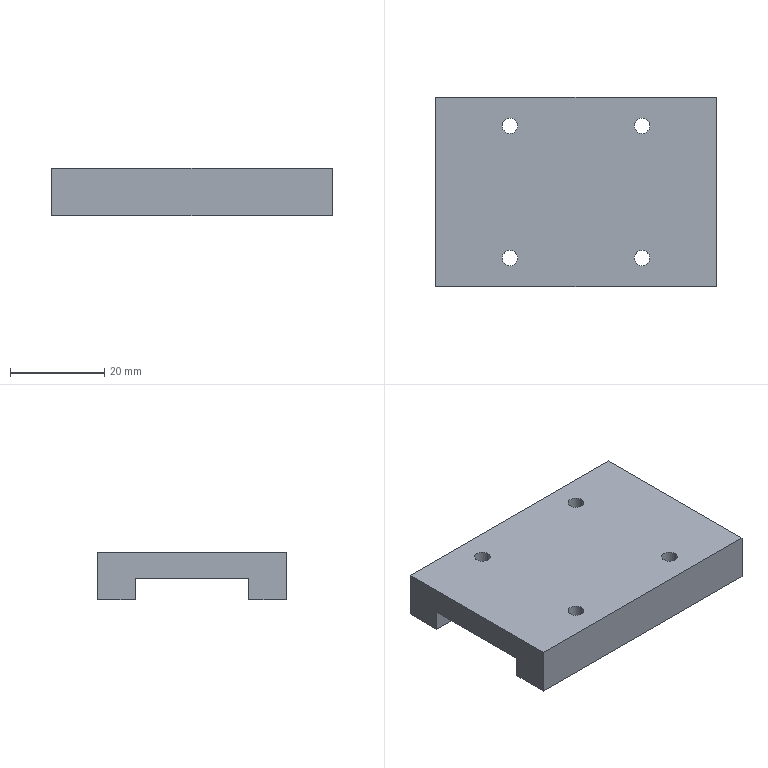Part | SolidWorks | features Extrusion 1, HoleWzd 1, ICE 1 | 1 solid | 18 faces | box 59.4 x 40 x 10 mm | volume 17003 mm3 | plane 10 | cylinder 8 | commonest cylinder face diameters 3.3 x8
STEP:
#1=CARTESIAN_POINT('',(-15.65,14.,0.));
#2=VERTEX_POINT('',#1);
#3=CARTESIAN_POINT('',(-12.35,14.,0.));
#4=VERTEX_POINT('',#3);
#5=CARTESIAN_POINT('',(-14.,14.,0.));
#6=DIRECTION('',(0.,0.,1.));
#7=DIRECTION('',(1.,0.,0.));
#8=AXIS2_PLACEMENT_3D('',#5,#6,#7);
#9=CIRCLE('',#8,1.65);
#10=EDGE_CURVE('',#2,#4,#9,.T.);
#11=ORIENTED_EDGE('',*,*,#10,.F.);
#12=CARTESIAN_POINT('',(-15.65,14.,10.));
#13=VERTEX_POINT('',#12);
#14=CARTESIAN_POINT('',(-15.65,14.,10.));
#15=DIRECTION('',(0.,0.,1.));
#16=VECTOR('',#15,1000.);
#17=LINE('',#14,#16);
#18=EDGE_CURVE('',#2,#13,#17,.T.);
#19=ORIENTED_EDGE('',*,*,#18,.T.);
#20=CARTESIAN_POINT('',(-12.35,14.,10.));
#21=VERTEX_POINT('',#20);
#22=CARTESIAN_POINT('',(-14.,14.,10.));
#23=DIRECTION('',(0.,0.,1.));
#24=DIRECTION('',(1.,0.,0.));
#25=AXIS2_PLACEMENT_3D('',#22,#23,#24);
#26=CIRCLE('',#25,1.65);
#27=EDGE_CURVE('',#13,#21,#26,.T.);
#28=ORIENTED_EDGE('',*,*,#27,.T.);
#29=CARTESIAN_POINT('',(-12.35,14.,10.));
#30=DIRECTION('',(0.,0.,1.));
#31=VECTOR('',#30,1000.);
#32=LINE('',#29,#31);
#33=EDGE_CURVE('',#4,#21,#32,.T.);
#34=ORIENTED_EDGE('',*,*,#33,.F.);
#35=EDGE_LOOP('',(#11,#19,#28,#34));
#36=FACE_OUTER_BOUND('',#35,.T.);
#37=CARTESIAN_POINT('',(-14.,14.,10.));
#38=DIRECTION('',(0.,0.,1.));
#39=DIRECTION('',(1.,0.,0.));
#40=AXIS2_PLACEMENT_3D('',#37,#38,#39);
#41=CYLINDRICAL_SURFACE('',#40,1.65);
#42=ADVANCED_FACE('',(#36),#41,.F.);
#43=CARTESIAN_POINT('',(12.35,14.,0.));
#44=VERTEX_POINT('',#43);
#45=CARTESIAN_POINT('',(15.65,14.,0.));
#46=VERTEX_POINT('',#45);
#47=CARTESIAN_POINT('',(14.,14.,0.));
#48=DIRECTION('',(0.,0.,1.));
#49=DIRECTION('',(1.,0.,0.));
#50=AXIS2_PLACEMENT_3D('',#47,#48,#49);
#51=CIRCLE('',#50,1.65);
#52=EDGE_CURVE('',#44,#46,#51,.T.);
#53=ORIENTED_EDGE('',*,*,#52,.F.);
#54=CARTESIAN_POINT('',(12.35,14.,10.));
#55=VERTEX_POINT('',#54);
#56=CARTESIAN_POINT('',(12.35,14.,10.));
#57=DIRECTION('',(0.,0.,1.));
#58=VECTOR('',#57,1000.);
#59=LINE('',#56,#58);
#60=EDGE_CURVE('',#44,#55,#59,.T.);
#61=ORIENTED_EDGE('',*,*,#60,.T.);
#62=CARTESIAN_POINT('',(15.65,14.,10.));
#63=VERTEX_POINT('',#62);
#64=CARTESIAN_POINT('',(14.,14.,10.));
#65=DIRECTION('',(0.,0.,1.));
#66=DIRECTION('',(1.,0.,0.));
#67=AXIS2_PLACEMENT_3D('',#64,#65,#66);
#68=CIRCLE('',#67,1.65);
#69=EDGE_CURVE('',#55,#63,#68,.T.);
#70=ORIENTED_EDGE('',*,*,#69,.T.);
#71=CARTESIAN_POINT('',(15.65,14.,10.));
#72=DIRECTION('',(0.,0.,1.));
#73=VECTOR('',#72,1000.);
#74=LINE('',#71,#73);
#75=EDGE_CURVE('',#46,#63,#74,.T.);
#76=ORIENTED_EDGE('',*,*,#75,.F.);
#77=EDGE_LOOP('',(#53,#61,#70,#76));
#78=FACE_OUTER_BOUND('',#77,.T.);
#79=CARTESIAN_POINT('',(14.,14.,10.));
#80=DIRECTION('',(0.,0.,1.));
#81=DIRECTION('',(1.,0.,0.));
#82=AXIS2_PLACEMENT_3D('',#79,#80,#81);
#83=CYLINDRICAL_SURFACE('',#82,1.65);
#84=ADVANCED_FACE('',(#78),#83,.F.);
#85=CARTESIAN_POINT('',(12.35,-14.,0.));
#86=VERTEX_POINT('',#85);
#87=CARTESIAN_POINT('',(15.65,-14.,0.));
#88=VERTEX_POINT('',#87);
#89=CARTESIAN_POINT('',(14.,-14.,0.));
#90=DIRECTION('',(0.,0.,1.));
#91=DIRECTION('',(1.,0.,0.));
#92=AXIS2_PLACEMENT_3D('',#89,#90,#91);
#93=CIRCLE('',#92,1.65);
#94=EDGE_CURVE('',#86,#88,#93,.T.);
#95=ORIENTED_EDGE('',*,*,#94,.F.);
#96=CARTESIAN_POINT('',(12.35,-14.,10.));
#97=VERTEX_POINT('',#96);
#98=CARTESIAN_POINT('',(12.35,-14.,10.));
#99=DIRECTION('',(0.,0.,1.));
#100=VECTOR('',#99,1000.);
#101=LINE('',#98,#100);
#102=EDGE_CURVE('',#86,#97,#101,.T.);
#103=ORIENTED_EDGE('',*,*,#102,.T.);
#104=CARTESIAN_POINT('',(15.65,-14.,10.));
#105=VERTEX_POINT('',#104);
#106=CARTESIAN_POINT('',(14.,-14.,10.));
#107=DIRECTION('',(0.,0.,1.));
#108=DIRECTION('',(1.,0.,0.));
#109=AXIS2_PLACEMENT_3D('',#106,#107,#108);
#110=CIRCLE('',#109,1.65);
#111=EDGE_CURVE('',#97,#105,#110,.T.);
#112=ORIENTED_EDGE('',*,*,#111,.T.);
#113=CARTESIAN_POINT('',(15.65,-14.,10.));
#114=DIRECTION('',(0.,0.,1.));
#115=VECTOR('',#114,1000.);
#116=LINE('',#113,#115);
#117=EDGE_CURVE('',#88,#105,#116,.T.);
#118=ORIENTED_EDGE('',*,*,#117,.F.);
#119=EDGE_LOOP('',(#95,#103,#112,#118));
#120=FACE_OUTER_BOUND('',#119,.T.);
#121=CARTESIAN_POINT('',(14.,-14.,10.));
#122=DIRECTION('',(0.,0.,1.));
#123=DIRECTION('',(1.,0.,0.));
#124=AXIS2_PLACEMENT_3D('',#121,#122,#123);
#125=CYLINDRICAL_SURFACE('',#124,1.65);
#126=ADVANCED_FACE('',(#120),#125,.F.);
#127=CARTESIAN_POINT('',(-15.65,-14.,0.));
#128=VERTEX_POINT('',#127);
#129=CARTESIAN_POINT('',(-12.35,-14.,0.));
#130=VERTEX_POINT('',#129);
#131=CARTESIAN_POINT('',(-14.,-14.,0.));
#132=DIRECTION('',(0.,0.,1.));
#133=DIRECTION('',(1.,0.,0.));
#134=AXIS2_PLACEMENT_3D('',#131,#132,#133);
#135=CIRCLE('',#134,1.65);
#136=EDGE_CURVE('',#128,#130,#135,.T.);
#137=ORIENTED_EDGE('',*,*,#136,.F.);
#138=CARTESIAN_POINT('',(-15.65,-14.,10.));
#139=VERTEX_POINT('',#138);
#140=CARTESIAN_POINT('',(-15.65,-14.,10.));
#141=DIRECTION('',(0.,0.,1.));
#142=VECTOR('',#141,1000.);
#143=LINE('',#140,#142);
#144=EDGE_CURVE('',#128,#139,#143,.T.);
#145=ORIENTED_EDGE('',*,*,#144,.T.);
#146=CARTESIAN_POINT('',(-12.35,-14.,10.));
#147=VERTEX_POINT('',#146);
#148=CARTESIAN_POINT('',(-14.,-14.,10.));
#149=DIRECTION('',(0.,0.,1.));
#150=DIRECTION('',(1.,0.,0.));
#151=AXIS2_PLACEMENT_3D('',#148,#149,#150);
#152=CIRCLE('',#151,1.65);
#153=EDGE_CURVE('',#139,#147,#152,.T.);
#154=ORIENTED_EDGE('',*,*,#153,.T.);
#155=CARTESIAN_POINT('',(-12.35,-14.,10.));
#156=DIRECTION('',(0.,0.,1.));
#157=VECTOR('',#156,1000.);
#158=LINE('',#155,#157);
#159=EDGE_CURVE('',#130,#147,#158,.T.);
#160=ORIENTED_EDGE('',*,*,#159,.F.);
#161=EDGE_LOOP('',(#137,#145,#154,#160));
#162=FACE_OUTER_BOUND('',#161,.T.);
#163=CARTESIAN_POINT('',(-14.,-14.,10.));
#164=DIRECTION('',(0.,0.,1.));
#165=DIRECTION('',(1.,0.,0.));
#166=AXIS2_PLACEMENT_3D('',#163,#164,#165);
#167=CYLINDRICAL_SURFACE('',#166,1.65);
#168=ADVANCED_FACE('',(#162),#167,.F.);
#169=CARTESIAN_POINT('',(14.,-14.,0.));
#170=DIRECTION('',(0.,0.,1.));
#171=DIRECTION('',(1.,0.,0.));
#172=AXIS2_PLACEMENT_3D('',#169,#170,#171);
#173=CIRCLE('',#172,1.65);
#174=EDGE_CURVE('',#88,#86,#173,.T.);
#175=ORIENTED_EDGE('',*,*,#174,.T.);
#176=ORIENTED_EDGE('',*,*,#94,.T.);
#177=EDGE_LOOP('',(#175,#176));
#178=FACE_BOUND('',#177,.T.);
#179=CARTESIAN_POINT('',(-14.,-14.,0.));
#180=DIRECTION('',(0.,0.,1.));
#181=DIRECTION('',(1.,0.,0.));
#182=AXIS2_PLACEMENT_3D('',#179,#180,#181);
#183=CIRCLE('',#182,1.65);
#184=EDGE_CURVE('',#130,#128,#183,.T.);
#185=ORIENTED_EDGE('',*,*,#184,.T.);
#186=ORIENTED_EDGE('',*,*,#136,.T.);
#187=EDGE_LOOP('',(#185,#186));
#188=FACE_BOUND('',#187,.T.);
#189=CARTESIAN_POINT('',(-29.7,-12.,0.));
#190=VERTEX_POINT('',#189);
#191=CARTESIAN_POINT('',(-29.7,-20.,0.));
#192=VERTEX_POINT('',#191);
#193=CARTESIAN_POINT('',(-29.7,20.,0.));
#194=DIRECTION('',(0.,-1.,0.));
#195=VECTOR('',#194,1000.);
#196=LINE('',#193,#195);
#197=EDGE_CURVE('',#190,#192,#196,.T.);
#198=ORIENTED_EDGE('',*,*,#197,.F.);
#199=CARTESIAN_POINT('',(29.7,-12.,0.));
#200=VERTEX_POINT('',#199);
#201=CARTESIAN_POINT('',(0.,-12.,0.));
#202=DIRECTION('',(1.,0.,0.));
#203=VECTOR('',#202,1000.);
#204=LINE('',#201,#203);
#205=EDGE_CURVE('',#190,#200,#204,.T.);
#206=ORIENTED_EDGE('',*,*,#205,.T.);
#207=CARTESIAN_POINT('',(29.7,-20.,0.));
#208=VERTEX_POINT('',#207);
#209=CARTESIAN_POINT('',(29.7,20.,0.));
#210=DIRECTION('',(0.,1.,0.));
#211=VECTOR('',#210,1000.);
#212=LINE('',#209,#211);
#213=EDGE_CURVE('',#208,#200,#212,.T.);
#214=ORIENTED_EDGE('',*,*,#213,.F.);
#215=CARTESIAN_POINT('',(-29.7,-20.,0.));
#216=DIRECTION('',(1.,0.,0.));
#217=VECTOR('',#216,1000.);
#218=LINE('',#215,#217);
#219=EDGE_CURVE('',#192,#208,#218,.T.);
#220=ORIENTED_EDGE('',*,*,#219,.F.);
#221=EDGE_LOOP('',(#198,#206,#214,#220));
#222=FACE_OUTER_BOUND('',#221,.T.);
#223=CARTESIAN_POINT('',(0.,0.,0.));
#224=DIRECTION('',(0.,0.,1.));
#225=DIRECTION('',(1.,0.,0.));
#226=AXIS2_PLACEMENT_3D('',#223,#224,#225);
#227=PLANE('',#226);
#228=ADVANCED_FACE('',(#178,#188,#222),#227,.F.);
#229=ORIENTED_EDGE('',*,*,#213,.T.);
#230=CARTESIAN_POINT('',(29.7,-12.,4.5));
#231=VERTEX_POINT('',#230);
#232=CARTESIAN_POINT('',(29.7,-12.,-4.5));
#233=DIRECTION('',(0.,0.,1.));
#234=VECTOR('',#233,1000.);
#235=LINE('',#232,#234);
#236=EDGE_CURVE('',#200,#231,#235,.T.);
#237=ORIENTED_EDGE('',*,*,#236,.T.);
#238=CARTESIAN_POINT('',(29.7,12.,4.5));
#239=VERTEX_POINT('',#238);
#240=CARTESIAN_POINT('',(29.7,12.,4.5));
#241=DIRECTION('',(0.,1.,0.));
#242=VECTOR('',#241,1000.);
#243=LINE('',#240,#242);
#244=EDGE_CURVE('',#231,#239,#243,.T.);
#245=ORIENTED_EDGE('',*,*,#244,.T.);
#246=CARTESIAN_POINT('',(29.7,12.,0.));
#247=VERTEX_POINT('',#246);
#248=CARTESIAN_POINT('',(29.7,12.,-4.5));
#249=DIRECTION('',(0.,0.,-1.));
#250=VECTOR('',#249,1000.);
#251=LINE('',#248,#250);
#252=EDGE_CURVE('',#239,#247,#251,.T.);
#253=ORIENTED_EDGE('',*,*,#252,.T.);
#254=CARTESIAN_POINT('',(29.7,20.,0.));
#255=VERTEX_POINT('',#254);
#256=CARTESIAN_POINT('',(29.7,20.,0.));
#257=DIRECTION('',(0.,1.,0.));
#258=VECTOR('',#257,1000.);
#259=LINE('',#256,#258);
#260=EDGE_CURVE('',#247,#255,#259,.T.);
#261=ORIENTED_EDGE('',*,*,#260,.T.);
#262=CARTESIAN_POINT('',(29.7,20.,10.));
#263=VERTEX_POINT('',#262);
#264=CARTESIAN_POINT('',(29.7,20.,10.));
#265=DIRECTION('',(0.,0.,-1.));
#266=VECTOR('',#265,1000.);
#267=LINE('',#264,#266);
#268=EDGE_CURVE('',#263,#255,#267,.T.);
#269=ORIENTED_EDGE('',*,*,#268,.F.);
#270=CARTESIAN_POINT('',(29.7,-20.,10.));
#271=VERTEX_POINT('',#270);
#272=CARTESIAN_POINT('',(29.7,20.,10.));
#273=DIRECTION('',(0.,1.,0.));
#274=VECTOR('',#273,1000.);
#275=LINE('',#272,#274);
#276=EDGE_CURVE('',#271,#263,#275,.T.);
#277=ORIENTED_EDGE('',*,*,#276,.F.);
#278=CARTESIAN_POINT('',(29.7,-20.,10.));
#279=DIRECTION('',(0.,0.,-1.));
#280=VECTOR('',#279,1000.);
#281=LINE('',#278,#280);
#282=EDGE_CURVE('',#271,#208,#281,.T.);
#283=ORIENTED_EDGE('',*,*,#282,.T.);
#284=EDGE_LOOP('',(#229,#237,#245,#253,#261,#269,#277,#283));
#285=FACE_OUTER_BOUND('',#284,.T.);
#286=CARTESIAN_POINT('',(29.7,20.,10.));
#287=DIRECTION('',(-1.,0.,0.));
#288=DIRECTION('',(0.,-1.,0.));
#289=AXIS2_PLACEMENT_3D('',#286,#287,#288);
#290=PLANE('',#289);
#291=ADVANCED_FACE('',(#285),#290,.F.);
#292=CARTESIAN_POINT('',(-29.7,20.,0.));
#293=VERTEX_POINT('',#292);
#294=CARTESIAN_POINT('',(-29.7,20.,0.));
#295=DIRECTION('',(-1.,0.,0.));
#296=VECTOR('',#295,1000.);
#297=LINE('',#294,#296);
#298=EDGE_CURVE('',#255,#293,#297,.T.);
#299=ORIENTED_EDGE('',*,*,#298,.T.);
#300=CARTESIAN_POINT('',(-29.7,20.,10.));
#301=VERTEX_POINT('',#300);
#302=CARTESIAN_POINT('',(-29.7,20.,10.));
#303=DIRECTION('',(0.,0.,-1.));
#304=VECTOR('',#303,1000.);
#305=LINE('',#302,#304);
#306=EDGE_CURVE('',#301,#293,#305,.T.);
#307=ORIENTED_EDGE('',*,*,#306,.F.);
#308=CARTESIAN_POINT('',(-29.7,20.,10.));
#309=DIRECTION('',(-1.,0.,0.));
#310=VECTOR('',#309,1000.);
#311=LINE('',#308,#310);
#312=EDGE_CURVE('',#263,#301,#311,.T.);
#313=ORIENTED_EDGE('',*,*,#312,.F.);
#314=ORIENTED_EDGE('',*,*,#268,.T.);
#315=EDGE_LOOP('',(#299,#307,#313,#314));
#316=FACE_OUTER_BOUND('',#315,.T.);
#317=CARTESIAN_POINT('',(-29.7,20.,10.));
#318=DIRECTION('',(0.,-1.,0.));
#319=DIRECTION('',(0.,0.,-1.));
#320=AXIS2_PLACEMENT_3D('',#317,#318,#319);
#321=PLANE('',#320);
#322=ADVANCED_FACE('',(#316),#321,.F.);
#323=CARTESIAN_POINT('',(-29.7,-12.,4.5));
#324=VERTEX_POINT('',#323);
#325=CARTESIAN_POINT('',(-29.7,12.,4.5));
#326=VERTEX_POINT('',#325);
#327=CARTESIAN_POINT('',(-29.7,12.,4.5));
#328=DIRECTION('',(0.,1.,0.));
#329=VECTOR('',#328,1000.);
#330=LINE('',#327,#329);
#331=EDGE_CURVE('',#324,#326,#330,.T.);
#332=ORIENTED_EDGE('',*,*,#331,.F.);
#333=CARTESIAN_POINT('',(-29.7,-12.,-4.5));
#334=DIRECTION('',(0.,0.,1.));
#335=VECTOR('',#334,1000.);
#336=LINE('',#333,#335);
#337=EDGE_CURVE('',#190,#324,#336,.T.);
#338=ORIENTED_EDGE('',*,*,#337,.F.);
#339=ORIENTED_EDGE('',*,*,#197,.T.);
#340=CARTESIAN_POINT('',(-29.7,-20.,10.));
#341=VERTEX_POINT('',#340);
#342=CARTESIAN_POINT('',(-29.7,-20.,10.));
#343=DIRECTION('',(0.,0.,-1.));
#344=VECTOR('',#343,1000.);
#345=LINE('',#342,#344);
#346=EDGE_CURVE('',#341,#192,#345,.T.);
#347=ORIENTED_EDGE('',*,*,#346,.F.);
#348=CARTESIAN_POINT('',(-29.7,20.,10.));
#349=DIRECTION('',(0.,-1.,0.));
#350=VECTOR('',#349,1000.);
#351=LINE('',#348,#350);
#352=EDGE_CURVE('',#301,#341,#351,.T.);
#353=ORIENTED_EDGE('',*,*,#352,.F.);
#354=ORIENTED_EDGE('',*,*,#306,.T.);
#355=CARTESIAN_POINT('',(-29.7,12.,0.));
#356=VERTEX_POINT('',#355);
#357=CARTESIAN_POINT('',(-29.7,20.,0.));
#358=DIRECTION('',(0.,-1.,0.));
#359=VECTOR('',#358,1000.);
#360=LINE('',#357,#359);
#361=EDGE_CURVE('',#293,#356,#360,.T.);
#362=ORIENTED_EDGE('',*,*,#361,.T.);
#363=CARTESIAN_POINT('',(-29.7,12.,-4.5));
#364=DIRECTION('',(0.,0.,-1.));
#365=VECTOR('',#364,1000.);
#366=LINE('',#363,#365);
#367=EDGE_CURVE('',#326,#356,#366,.T.);
#368=ORIENTED_EDGE('',*,*,#367,.F.);
#369=EDGE_LOOP('',(#332,#338,#339,#347,#353,#354,#362,#368));
#370=FACE_OUTER_BOUND('',#369,.T.);
#371=CARTESIAN_POINT('',(-29.7,20.,10.));
#372=DIRECTION('',(1.,0.,0.));
#373=DIRECTION('',(0.,1.,0.));
#374=AXIS2_PLACEMENT_3D('',#371,#372,#373);
#375=PLANE('',#374);
#376=ADVANCED_FACE('',(#370),#375,.F.);
#377=ORIENTED_EDGE('',*,*,#219,.T.);
#378=ORIENTED_EDGE('',*,*,#282,.F.);
#379=CARTESIAN_POINT('',(-29.7,-20.,10.));
#380=DIRECTION('',(1.,0.,0.));
#381=VECTOR('',#380,1000.);
#382=LINE('',#379,#381);
#383=EDGE_CURVE('',#341,#271,#382,.T.);
#384=ORIENTED_EDGE('',*,*,#383,.F.);
#385=ORIENTED_EDGE('',*,*,#346,.T.);
#386=EDGE_LOOP('',(#377,#378,#384,#385));
#387=FACE_OUTER_BOUND('',#386,.T.);
#388=CARTESIAN_POINT('',(-29.7,-20.,10.));
#389=DIRECTION('',(0.,1.,0.));
#390=DIRECTION('',(0.,0.,1.));
#391=AXIS2_PLACEMENT_3D('',#388,#389,#390);
#392=PLANE('',#391);
#393=ADVANCED_FACE('',(#387),#392,.F.);
#394=CARTESIAN_POINT('',(-14.,14.,10.));
#395=DIRECTION('',(0.,0.,1.));
#396=DIRECTION('',(1.,0.,0.));
#397=AXIS2_PLACEMENT_3D('',#394,#395,#396);
#398=CIRCLE('',#397,1.65);
#399=EDGE_CURVE('',#21,#13,#398,.T.);
#400=ORIENTED_EDGE('',*,*,#399,.F.);
#401=ORIENTED_EDGE('',*,*,#27,.F.);
#402=EDGE_LOOP('',(#400,#401));
#403=FACE_BOUND('',#402,.T.);
#404=CARTESIAN_POINT('',(14.,14.,10.));
#405=DIRECTION('',(0.,0.,1.));
#406=DIRECTION('',(1.,0.,0.));
#407=AXIS2_PLACEMENT_3D('',#404,#405,#406);
#408=CIRCLE('',#407,1.65);
#409=EDGE_CURVE('',#63,#55,#408,.T.);
#410=ORIENTED_EDGE('',*,*,#409,.F.);
#411=ORIENTED_EDGE('',*,*,#69,.F.);
#412=EDGE_LOOP('',(#410,#411));
#413=FACE_BOUND('',#412,.T.);
#414=CARTESIAN_POINT('',(14.,-14.,10.));
#415=DIRECTION('',(0.,0.,1.));
#416=DIRECTION('',(1.,0.,0.));
#417=AXIS2_PLACEMENT_3D('',#414,#415,#416);
#418=CIRCLE('',#417,1.65);
#419=EDGE_CURVE('',#105,#97,#418,.T.);
#420=ORIENTED_EDGE('',*,*,#419,.F.);
#421=ORIENTED_EDGE('',*,*,#111,.F.);
#422=EDGE_LOOP('',(#420,#421));
#423=FACE_BOUND('',#422,.T.);
#424=CARTESIAN_POINT('',(-14.,-14.,10.));
#425=DIRECTION('',(0.,0.,1.));
#426=DIRECTION('',(1.,0.,0.));
#427=AXIS2_PLACEMENT_3D('',#424,#425,#426);
#428=CIRCLE('',#427,1.65);
#429=EDGE_CURVE('',#147,#139,#428,.T.);
#430=ORIENTED_EDGE('',*,*,#429,.F.);
#431=ORIENTED_EDGE('',*,*,#153,.F.);
#432=EDGE_LOOP('',(#430,#431));
#433=FACE_BOUND('',#432,.T.);
#434=ORIENTED_EDGE('',*,*,#276,.T.);
#435=ORIENTED_EDGE('',*,*,#312,.T.);
#436=ORIENTED_EDGE('',*,*,#352,.T.);
#437=ORIENTED_EDGE('',*,*,#383,.T.);
#438=EDGE_LOOP('',(#434,#435,#436,#437));
#439=FACE_OUTER_BOUND('',#438,.T.);
#440=CARTESIAN_POINT('',(0.,0.,10.));
#441=DIRECTION('',(0.,0.,1.));
#442=DIRECTION('',(1.,0.,0.));
#443=AXIS2_PLACEMENT_3D('',#440,#441,#442);
#444=PLANE('',#443);
#445=ADVANCED_FACE('',(#403,#413,#423,#433,#439),#444,.T.);
#446=CARTESIAN_POINT('',(-14.,14.,0.));
#447=DIRECTION('',(0.,0.,1.));
#448=DIRECTION('',(1.,0.,0.));
#449=AXIS2_PLACEMENT_3D('',#446,#447,#448);
#450=CIRCLE('',#449,1.65);
#451=EDGE_CURVE('',#4,#2,#450,.T.);
#452=ORIENTED_EDGE('',*,*,#451,.T.);
#453=ORIENTED_EDGE('',*,*,#10,.T.);
#454=EDGE_LOOP('',(#452,#453));
#455=FACE_BOUND('',#454,.T.);
#456=CARTESIAN_POINT('',(14.,14.,0.));
#457=DIRECTION('',(0.,0.,1.));
#458=DIRECTION('',(1.,0.,0.));
#459=AXIS2_PLACEMENT_3D('',#456,#457,#458);
#460=CIRCLE('',#459,1.65);
#461=EDGE_CURVE('',#46,#44,#460,.T.);
#462=ORIENTED_EDGE('',*,*,#461,.T.);
#463=ORIENTED_EDGE('',*,*,#52,.T.);
#464=EDGE_LOOP('',(#462,#463));
#465=FACE_BOUND('',#464,.T.);
#466=ORIENTED_EDGE('',*,*,#260,.F.);
#467=CARTESIAN_POINT('',(0.,12.,0.));
#468=DIRECTION('',(-1.,0.,0.));
#469=VECTOR('',#468,1000.);
#470=LINE('',#467,#469);
#471=EDGE_CURVE('',#247,#356,#470,.T.);
#472=ORIENTED_EDGE('',*,*,#471,.T.);
#473=ORIENTED_EDGE('',*,*,#361,.F.);
#474=ORIENTED_EDGE('',*,*,#298,.F.);
#475=EDGE_LOOP('',(#466,#472,#473,#474));
#476=FACE_OUTER_BOUND('',#475,.T.);
#477=CARTESIAN_POINT('',(0.,0.,0.));
#478=DIRECTION('',(0.,0.,1.));
#479=DIRECTION('',(1.,0.,0.));
#480=AXIS2_PLACEMENT_3D('',#477,#478,#479);
#481=PLANE('',#480);
#482=ADVANCED_FACE('',(#455,#465,#476),#481,.F.);
#483=ORIENTED_EDGE('',*,*,#337,.T.);
#484=CARTESIAN_POINT('',(29.7,-12.,4.5));
#485=DIRECTION('',(-1.,0.,0.));
#486=VECTOR('',#485,1000.);
#487=LINE('',#484,#486);
#488=EDGE_CURVE('',#231,#324,#487,.T.);
#489=ORIENTED_EDGE('',*,*,#488,.F.);
#490=ORIENTED_EDGE('',*,*,#236,.F.);
#491=ORIENTED_EDGE('',*,*,#205,.F.);
#492=EDGE_LOOP('',(#483,#489,#490,#491));
#493=FACE_OUTER_BOUND('',#492,.T.);
#494=CARTESIAN_POINT('',(29.7,-12.,-4.5));
#495=DIRECTION('',(0.,-1.,0.));
#496=DIRECTION('',(1.,0.,0.));
#497=AXIS2_PLACEMENT_3D('',#494,#495,#496);
#498=PLANE('',#497);
#499=ADVANCED_FACE('',(#493),#498,.F.);
#500=ORIENTED_EDGE('',*,*,#252,.F.);
#501=CARTESIAN_POINT('',(29.7,12.,4.5));
#502=DIRECTION('',(-1.,0.,0.));
#503=VECTOR('',#502,1000.);
#504=LINE('',#501,#503);
#505=EDGE_CURVE('',#239,#326,#504,.T.);
#506=ORIENTED_EDGE('',*,*,#505,.T.);
#507=ORIENTED_EDGE('',*,*,#367,.T.);
#508=ORIENTED_EDGE('',*,*,#471,.F.);
#509=EDGE_LOOP('',(#500,#506,#507,#508));
#510=FACE_OUTER_BOUND('',#509,.T.);
#511=CARTESIAN_POINT('',(29.7,12.,-4.5));
#512=DIRECTION('',(0.,1.,0.));
#513=DIRECTION('',(-1.,0.,0.));
#514=AXIS2_PLACEMENT_3D('',#511,#512,#513);
#515=PLANE('',#514);
#516=ADVANCED_FACE('',(#510),#515,.F.);
#517=ORIENTED_EDGE('',*,*,#331,.T.);
#518=ORIENTED_EDGE('',*,*,#505,.F.);
#519=ORIENTED_EDGE('',*,*,#244,.F.);
#520=ORIENTED_EDGE('',*,*,#488,.T.);
#521=EDGE_LOOP('',(#517,#518,#519,#520));
#522=FACE_OUTER_BOUND('',#521,.T.);
#523=CARTESIAN_POINT('',(29.7,12.,4.5));
#524=DIRECTION('',(0.,0.,1.));
#525=DIRECTION('',(1.,0.,0.));
#526=AXIS2_PLACEMENT_3D('',#523,#524,#525);
#527=PLANE('',#526);
#528=ADVANCED_FACE('',(#522),#527,.F.);
#529=ORIENTED_EDGE('',*,*,#144,.F.);
#530=ORIENTED_EDGE('',*,*,#184,.F.);
#531=ORIENTED_EDGE('',*,*,#159,.T.);
#532=ORIENTED_EDGE('',*,*,#429,.T.);
#533=EDGE_LOOP('',(#529,#530,#531,#532));
#534=FACE_OUTER_BOUND('',#533,.T.);
#535=CARTESIAN_POINT('',(-14.,-14.,10.));
#536=DIRECTION('',(0.,0.,1.));
#537=DIRECTION('',(1.,0.,0.));
#538=AXIS2_PLACEMENT_3D('',#535,#536,#537);
#539=CYLINDRICAL_SURFACE('',#538,1.65);
#540=ADVANCED_FACE('',(#534),#539,.F.);
#541=ORIENTED_EDGE('',*,*,#102,.F.);
#542=ORIENTED_EDGE('',*,*,#174,.F.);
#543=ORIENTED_EDGE('',*,*,#117,.T.);
#544=ORIENTED_EDGE('',*,*,#419,.T.);
#545=EDGE_LOOP('',(#541,#542,#543,#544));
#546=FACE_OUTER_BOUND('',#545,.T.);
#547=CARTESIAN_POINT('',(14.,-14.,10.));
#548=DIRECTION('',(0.,0.,1.));
#549=DIRECTION('',(1.,0.,0.));
#550=AXIS2_PLACEMENT_3D('',#547,#548,#549);
#551=CYLINDRICAL_SURFACE('',#550,1.65);
#552=ADVANCED_FACE('',(#546),#551,.F.);
#553=ORIENTED_EDGE('',*,*,#60,.F.);
#554=ORIENTED_EDGE('',*,*,#461,.F.);
#555=ORIENTED_EDGE('',*,*,#75,.T.);
#556=ORIENTED_EDGE('',*,*,#409,.T.);
#557=EDGE_LOOP('',(#553,#554,#555,#556));
#558=FACE_OUTER_BOUND('',#557,.T.);
#559=CARTESIAN_POINT('',(14.,14.,10.));
#560=DIRECTION('',(0.,0.,1.));
#561=DIRECTION('',(1.,0.,0.));
#562=AXIS2_PLACEMENT_3D('',#559,#560,#561);
#563=CYLINDRICAL_SURFACE('',#562,1.65);
#564=ADVANCED_FACE('',(#558),#563,.F.);
#565=ORIENTED_EDGE('',*,*,#18,.F.);
#566=ORIENTED_EDGE('',*,*,#451,.F.);
#567=ORIENTED_EDGE('',*,*,#33,.T.);
#568=ORIENTED_EDGE('',*,*,#399,.T.);
#569=EDGE_LOOP('',(#565,#566,#567,#568));
#570=FACE_OUTER_BOUND('',#569,.T.);
#571=CARTESIAN_POINT('',(-14.,14.,10.));
#572=DIRECTION('',(0.,0.,1.));
#573=DIRECTION('',(1.,0.,0.));
#574=AXIS2_PLACEMENT_3D('',#571,#572,#573);
#575=CYLINDRICAL_SURFACE('',#574,1.65);
#576=ADVANCED_FACE('',(#570),#575,.F.);
#577=CLOSED_SHELL('',(#42,#84,#126,#168,#228,#291,#322,#376,#393,#445,#482,#499,#516,#528,#540,#552,#564,#576));
#578=MANIFOLD_SOLID_BREP('',#577);
#579=CARTESIAN_POINT('',(0.,0.,0.));
#580=DIRECTION('',(0.,0.,1.));
#581=DIRECTION('',(1.,0.,0.));
#582=AXIS2_PLACEMENT_3D('',#579,#580,#581);
#583=(LENGTH_UNIT()NAMED_UNIT(*)SI_UNIT(.MILLI.,.METRE.));
#584=UNCERTAINTY_MEASURE_WITH_UNIT(LENGTH_MEASURE(0.00001),#583,'','');
#585=(NAMED_UNIT(*)PLANE_ANGLE_UNIT()SI_UNIT($,.RADIAN.));
#586=(NAMED_UNIT(*)SI_UNIT($,.STERADIAN.)SOLID_ANGLE_UNIT());
#587=(GEOMETRIC_REPRESENTATION_CONTEXT(3)GLOBAL_UNCERTAINTY_ASSIGNED_CONTEXT((#584))GLOBAL_UNIT_ASSIGNED_CONTEXT((#583,#585,#586))REPRESENTATION_CONTEXT('',''));
#588=ADVANCED_BREP_SHAPE_REPRESENTATION('',(#578,#582),#587);